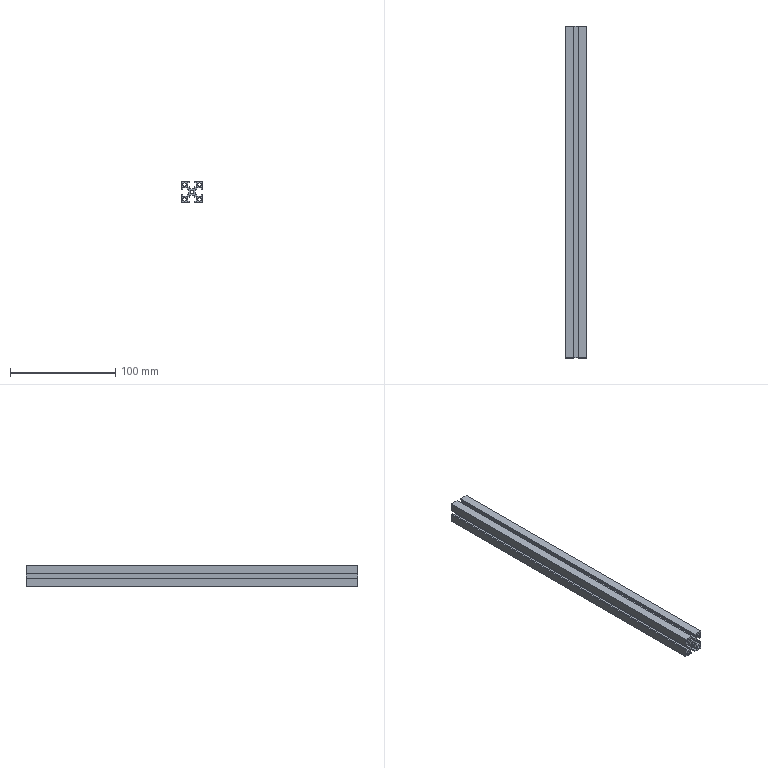Part | STEP file | 20 aluminium profile longitudinal 5 | 1 solid | 64 faces | box 20 x 316 x 20 mm | volume 56178 mm3 | plane 54 | cylinder 10 | commonest cylinder face diameters 3.3 x10